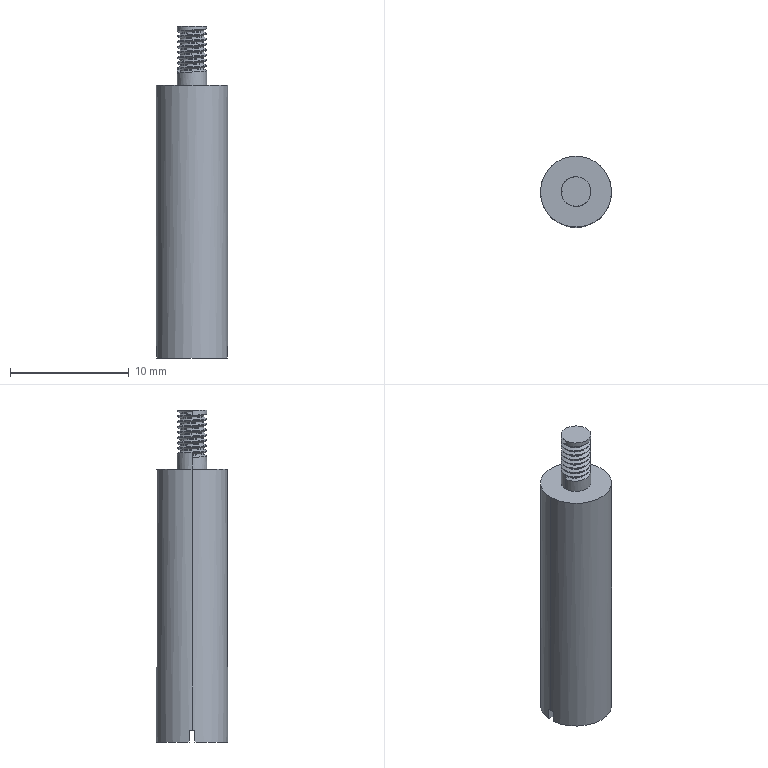Part | SolidWorks | features ICE 3, RevCut 2, Extrusion 1, Helix 1, RefAxis 1, SweepThread 1 | 1 solid | 41 faces | box 6 x 6 x 28 mm | volume 660.837 mm3 | cylinder 22 | plane 12 | cone 4 | spline 3 | commonest cylinder face diameters 2.5 x18 1.6 x2 6 x2